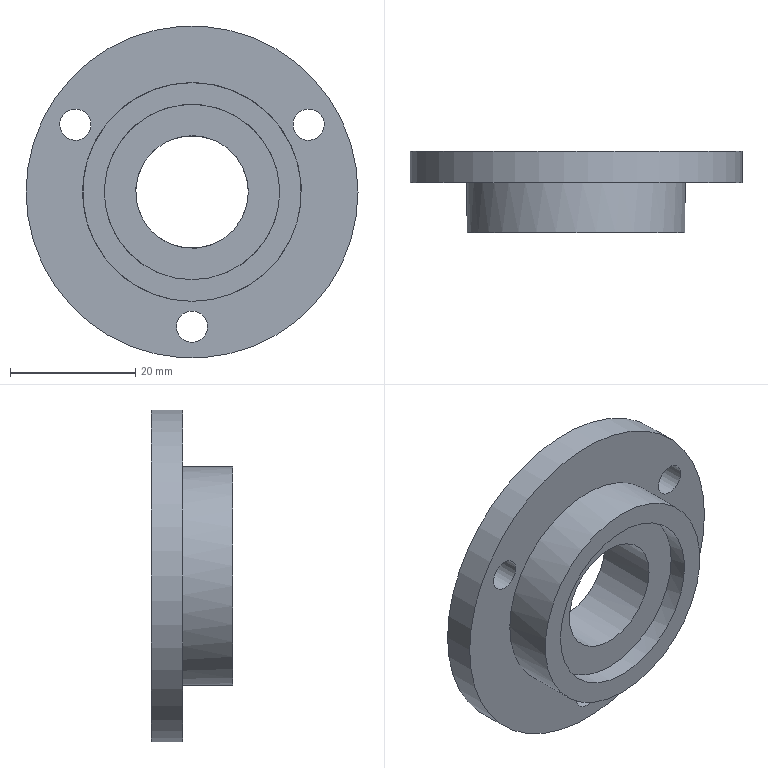Part | STEP file | YBQDJ-PD-19 | 1 solid | 11 faces | box 53 x 13 x 53 mm | volume 13997 mm3 | cylinder 7 | plane 4 | commonest cylinder face diameters 5 x3 18 x1 28 x1 34.9 x1 53 x1
STEP:
#1=CARTESIAN_POINT('',(0.,0.,0.));
#2=DIRECTION('',(0.,0.,1.));
#3=DIRECTION('',(1.,0.,0.));
#4=AXIS2_PLACEMENT_3D('',#1,#2,#3);
#5=CARTESIAN_POINT('',(-200.87,415.,131.915));
#6=VERTEX_POINT('',#5);
#7=CARTESIAN_POINT('',(-202.12,415.,129.75));
#8=DIRECTION('',(0.,1.,0.));
#9=DIRECTION('',(0.5,0.,0.866));
#10=AXIS2_PLACEMENT_3D('',#7,#8,#9);
#11=CIRCLE('',#10,2.5);
#12=CARTESIAN_POINT('',(-202.12,450.,129.75));
#13=DIRECTION('',(0.,-1.,0.));
#14=DIRECTION('',(-0.866,0.,0.5));
#15=AXIS2_PLACEMENT_3D('',#12,#13,#14);
#16=CYLINDRICAL_SURFACE('',#15,2.5);
#17=CARTESIAN_POINT('',(10.996,35.));
#18=DIRECTION('',(-1.,0.));
#19=VECTOR('',#18,1.);
#20=LINE('',#17,#19);
#21=(GEOMETRIC_REPRESENTATION_CONTEXT(2)PARAMETRIC_REPRESENTATION_CONTEXT()REPRESENTATION_CONTEXT('',''));
#22=DEFINITIONAL_REPRESENTATION('',(#20),#21);
#23=PCURVE('',#16,#22);
#24=CARTESIAN_POINT('',(-531.5,415.,22.));
#25=DIRECTION('',(0.,1.,0.));
#26=DIRECTION('',(0.,0.,-1.));
#27=AXIS2_PLACEMENT_3D('',#24,#25,#26);
#28=PLANE('',#27);
#29=CARTESIAN_POINT('',(-107.75,-329.38));
#30=DIRECTION('',(-0.866,-0.5));
#31=AXIS2_PLACEMENT_2D('',#29,#30);
#32=CIRCLE('',#31,2.5);
#33=(GEOMETRIC_REPRESENTATION_CONTEXT(2)PARAMETRIC_REPRESENTATION_CONTEXT()REPRESENTATION_CONTEXT('',''));
#34=DEFINITIONAL_REPRESENTATION('',(#32),#33);
#35=PCURVE('',#28,#34);
#36=SURFACE_CURVE('',#11,(#23,#35),.PCURVE_S1.);
#37=EDGE_CURVE('',#6,#6,#36,.T.);
#38=ORIENTED_EDGE('',*,*,#37,.T.);
#39=CARTESIAN_POINT('',(-200.87,420.,131.915));
#40=VERTEX_POINT('',#39);
#41=CARTESIAN_POINT('',(-200.87,420.,131.915));
#42=CARTESIAN_POINT('',(-200.87,415.,131.915));
#43=B_SPLINE_CURVE_WITH_KNOTS('',1,(#41,#42),.UNSPECIFIED.,.F.,.F.,(2,2),(30.,35.),.PIECEWISE_BEZIER_KNOTS.);
#44=CARTESIAN_POINT('',(4.712,0.));
#45=DIRECTION('',(0.,1.));
#46=VECTOR('',#45,1.);
#47=LINE('',#44,#46);
#48=(GEOMETRIC_REPRESENTATION_CONTEXT(2)PARAMETRIC_REPRESENTATION_CONTEXT()REPRESENTATION_CONTEXT('',''));
#49=DEFINITIONAL_REPRESENTATION('',(#47),#48);
#50=PCURVE('',#16,#49);
#51=CARTESIAN_POINT('',(10.996,0.));
#52=DIRECTION('',(0.,1.));
#53=VECTOR('',#52,1.);
#54=LINE('',#51,#53);
#55=(GEOMETRIC_REPRESENTATION_CONTEXT(2)PARAMETRIC_REPRESENTATION_CONTEXT()REPRESENTATION_CONTEXT('',''));
#56=DEFINITIONAL_REPRESENTATION('',(#54),#55);
#57=PCURVE('',#16,#56);
#58=SEAM_CURVE('',#43,(#50,#57),.PCURVE_S1.);
#59=EDGE_CURVE('',#40,#6,#58,.T.);
#60=ORIENTED_EDGE('',*,*,#59,.F.);
#61=CARTESIAN_POINT('',(-203.37,420.,127.585));
#62=VERTEX_POINT('',#61);
#63=CARTESIAN_POINT('',(-202.12,420.,129.75));
#64=DIRECTION('',(0.,1.,0.));
#65=DIRECTION('',(-0.5,0.,-0.866));
#66=AXIS2_PLACEMENT_3D('',#63,#64,#65);
#67=CIRCLE('',#66,2.5);
#68=CARTESIAN_POINT('',(7.854,30.));
#69=DIRECTION('',(-1.,0.));
#70=VECTOR('',#69,1.);
#71=LINE('',#68,#70);
#72=(GEOMETRIC_REPRESENTATION_CONTEXT(2)PARAMETRIC_REPRESENTATION_CONTEXT()REPRESENTATION_CONTEXT('',''));
#73=DEFINITIONAL_REPRESENTATION('',(#71),#72);
#74=PCURVE('',#16,#73);
#75=CARTESIAN_POINT('',(-183.5,420.,119.));
#76=DIRECTION('',(0.,-1.,0.));
#77=DIRECTION('',(-0.7071,0.,-0.7071));
#78=AXIS2_PLACEMENT_3D('',#75,#76,#77);
#79=PLANE('',#78);
#80=CARTESIAN_POINT('',(7.979,-20.12));
#81=CARTESIAN_POINT('',(9.1,-24.303));
#82=CARTESIAN_POINT('',(4.918,-23.182));
#83=CARTESIAN_POINT('',(0.735,-22.062));
#84=CARTESIAN_POINT('',(3.797,-19.));
#85=CARTESIAN_POINT('',(6.859,-15.938));
#86=CARTESIAN_POINT('',(7.979,-20.12));
#87=(BOUNDED_CURVE()B_SPLINE_CURVE(2,(#80,#81,#82,#83,#84,#85,#86),.UNSPECIFIED.,.T.,.F.)B_SPLINE_CURVE_WITH_KNOTS((1,2,2,2,2,1),(-2.094,0.,2.094,4.189,6.283,8.378),.UNSPECIFIED.)CURVE()GEOMETRIC_REPRESENTATION_ITEM()RATIONAL_B_SPLINE_CURVE((1.,0.5,1.,0.5,1.,0.5,1.))REPRESENTATION_ITEM(''));
#88=(GEOMETRIC_REPRESENTATION_CONTEXT(2)PARAMETRIC_REPRESENTATION_CONTEXT()REPRESENTATION_CONTEXT('',''));
#89=DEFINITIONAL_REPRESENTATION('',(#87),#88);
#90=PCURVE('',#79,#89);
#91=SURFACE_CURVE('',#67,(#74,#90),.PCURVE_S1.);
#92=EDGE_CURVE('',#62,#40,#91,.T.);
#93=ORIENTED_EDGE('',*,*,#92,.F.);
#94=CARTESIAN_POINT('',(-202.12,420.,129.75));
#95=DIRECTION('',(0.,1.,0.));
#96=DIRECTION('',(-0.5,0.,-0.866));
#97=AXIS2_PLACEMENT_3D('',#94,#95,#96);
#98=CIRCLE('',#97,2.5);
#99=CARTESIAN_POINT('',(14.137,30.));
#100=DIRECTION('',(-1.,0.));
#101=VECTOR('',#100,1.);
#102=LINE('',#99,#101);
#103=(GEOMETRIC_REPRESENTATION_CONTEXT(2)PARAMETRIC_REPRESENTATION_CONTEXT()REPRESENTATION_CONTEXT('',''));
#104=DEFINITIONAL_REPRESENTATION('',(#102),#103);
#105=PCURVE('',#16,#104);
#106=CARTESIAN_POINT('',(7.979,-20.12));
#107=CARTESIAN_POINT('',(9.1,-24.303));
#108=CARTESIAN_POINT('',(4.918,-23.182));
#109=CARTESIAN_POINT('',(0.735,-22.062));
#110=CARTESIAN_POINT('',(3.797,-19.));
#111=CARTESIAN_POINT('',(6.859,-15.938));
#112=CARTESIAN_POINT('',(7.979,-20.12));
#113=(BOUNDED_CURVE()B_SPLINE_CURVE(2,(#106,#107,#108,#109,#110,#111,#112),.UNSPECIFIED.,.T.,.F.)B_SPLINE_CURVE_WITH_KNOTS((1,2,2,2,2,1),(-2.094,0.,2.094,4.189,6.283,8.378),.UNSPECIFIED.)CURVE()GEOMETRIC_REPRESENTATION_ITEM()RATIONAL_B_SPLINE_CURVE((1.,0.5,1.,0.5,1.,0.5,1.))REPRESENTATION_ITEM(''));
#114=(GEOMETRIC_REPRESENTATION_CONTEXT(2)PARAMETRIC_REPRESENTATION_CONTEXT()REPRESENTATION_CONTEXT('',''));
#115=DEFINITIONAL_REPRESENTATION('',(#113),#114);
#116=PCURVE('',#79,#115);
#117=SURFACE_CURVE('',#98,(#105,#116),.PCURVE_S1.);
#118=EDGE_CURVE('',#40,#62,#117,.T.);
#119=ORIENTED_EDGE('',*,*,#118,.F.);
#120=ORIENTED_EDGE('',*,*,#59,.T.);
#121=EDGE_LOOP('',(#38,#60,#93,#119,#120));
#122=FACE_BOUND('',#121,.F.);
#123=ADVANCED_FACE('',(#122),#16,.F.);
#124=CARTESIAN_POINT('',(-163.63,415.,127.585));
#125=VERTEX_POINT('',#124);
#126=CARTESIAN_POINT('',(-164.88,415.,129.75));
#127=DIRECTION('',(0.,1.,0.));
#128=DIRECTION('',(0.5,0.,-0.866));
#129=AXIS2_PLACEMENT_3D('',#126,#127,#128);
#130=CIRCLE('',#129,2.5);
#131=CARTESIAN_POINT('',(-164.88,450.,129.75));
#132=DIRECTION('',(0.,-1.,0.));
#133=DIRECTION('',(0.866,0.,0.5));
#134=AXIS2_PLACEMENT_3D('',#131,#132,#133);
#135=CYLINDRICAL_SURFACE('',#134,2.5);
#136=CARTESIAN_POINT('',(10.996,35.));
#137=DIRECTION('',(-1.,0.));
#138=VECTOR('',#137,1.);
#139=LINE('',#136,#138);
#140=(GEOMETRIC_REPRESENTATION_CONTEXT(2)PARAMETRIC_REPRESENTATION_CONTEXT()REPRESENTATION_CONTEXT('',''));
#141=DEFINITIONAL_REPRESENTATION('',(#139),#140);
#142=PCURVE('',#135,#141);
#143=CARTESIAN_POINT('',(-107.75,-366.62));
#144=DIRECTION('',(0.866,-0.5));
#145=AXIS2_PLACEMENT_2D('',#143,#144);
#146=CIRCLE('',#145,2.5);
#147=(GEOMETRIC_REPRESENTATION_CONTEXT(2)PARAMETRIC_REPRESENTATION_CONTEXT()REPRESENTATION_CONTEXT('',''));
#148=DEFINITIONAL_REPRESENTATION('',(#146),#147);
#149=PCURVE('',#28,#148);
#150=SURFACE_CURVE('',#130,(#142,#149),.PCURVE_S1.);
#151=EDGE_CURVE('',#125,#125,#150,.T.);
#152=ORIENTED_EDGE('',*,*,#151,.T.);
#153=CARTESIAN_POINT('',(-163.63,420.,127.585));
#154=VERTEX_POINT('',#153);
#155=CARTESIAN_POINT('',(-163.63,420.,127.585));
#156=CARTESIAN_POINT('',(-163.63,415.,127.585));
#157=B_SPLINE_CURVE_WITH_KNOTS('',1,(#155,#156),.UNSPECIFIED.,.F.,.F.,(2,2),(30.,35.),.PIECEWISE_BEZIER_KNOTS.);
#158=CARTESIAN_POINT('',(4.712,0.));
#159=DIRECTION('',(0.,1.));
#160=VECTOR('',#159,1.);
#161=LINE('',#158,#160);
#162=(GEOMETRIC_REPRESENTATION_CONTEXT(2)PARAMETRIC_REPRESENTATION_CONTEXT()REPRESENTATION_CONTEXT('',''));
#163=DEFINITIONAL_REPRESENTATION('',(#161),#162);
#164=PCURVE('',#135,#163);
#165=CARTESIAN_POINT('',(10.996,0.));
#166=DIRECTION('',(0.,1.));
#167=VECTOR('',#166,1.);
#168=LINE('',#165,#167);
#169=(GEOMETRIC_REPRESENTATION_CONTEXT(2)PARAMETRIC_REPRESENTATION_CONTEXT()REPRESENTATION_CONTEXT('',''));
#170=DEFINITIONAL_REPRESENTATION('',(#168),#169);
#171=PCURVE('',#135,#170);
#172=SEAM_CURVE('',#157,(#164,#171),.PCURVE_S1.);
#173=EDGE_CURVE('',#154,#125,#172,.T.);
#174=ORIENTED_EDGE('',*,*,#173,.F.);
#175=CARTESIAN_POINT('',(-166.13,420.,131.915));
#176=VERTEX_POINT('',#175);
#177=CARTESIAN_POINT('',(-164.88,420.,129.75));
#178=DIRECTION('',(0.,1.,0.));
#179=DIRECTION('',(-0.5,0.,0.866));
#180=AXIS2_PLACEMENT_3D('',#177,#178,#179);
#181=CIRCLE('',#180,2.5);
#182=CARTESIAN_POINT('',(7.854,30.));
#183=DIRECTION('',(-1.,0.));
#184=VECTOR('',#183,1.);
#185=LINE('',#182,#184);
#186=(GEOMETRIC_REPRESENTATION_CONTEXT(2)PARAMETRIC_REPRESENTATION_CONTEXT()REPRESENTATION_CONTEXT('',''));
#187=DEFINITIONAL_REPRESENTATION('',(#185),#186);
#188=PCURVE('',#135,#187);
#189=CARTESIAN_POINT('',(-21.414,3.15));
#190=CARTESIAN_POINT('',(-25.597,4.271));
#191=CARTESIAN_POINT('',(-22.535,7.332));
#192=CARTESIAN_POINT('',(-19.473,10.394));
#193=CARTESIAN_POINT('',(-18.353,6.212));
#194=CARTESIAN_POINT('',(-17.232,2.029));
#195=CARTESIAN_POINT('',(-21.414,3.15));
#196=(BOUNDED_CURVE()B_SPLINE_CURVE(2,(#189,#190,#191,#192,#193,#194,#195),.UNSPECIFIED.,.T.,.F.)B_SPLINE_CURVE_WITH_KNOTS((1,2,2,2,2,1),(-2.094,0.,2.094,4.189,6.283,8.378),.UNSPECIFIED.)CURVE()GEOMETRIC_REPRESENTATION_ITEM()RATIONAL_B_SPLINE_CURVE((1.,0.5,1.,0.5,1.,0.5,1.))REPRESENTATION_ITEM(''));
#197=(GEOMETRIC_REPRESENTATION_CONTEXT(2)PARAMETRIC_REPRESENTATION_CONTEXT()REPRESENTATION_CONTEXT('',''));
#198=DEFINITIONAL_REPRESENTATION('',(#196),#197);
#199=PCURVE('',#79,#198);
#200=SURFACE_CURVE('',#181,(#188,#199),.PCURVE_S1.);
#201=EDGE_CURVE('',#176,#154,#200,.T.);
#202=ORIENTED_EDGE('',*,*,#201,.F.);
#203=CARTESIAN_POINT('',(-164.88,420.,129.75));
#204=DIRECTION('',(0.,1.,0.));
#205=DIRECTION('',(-0.5,0.,0.866));
#206=AXIS2_PLACEMENT_3D('',#203,#204,#205);
#207=CIRCLE('',#206,2.5);
#208=CARTESIAN_POINT('',(14.137,30.));
#209=DIRECTION('',(-1.,0.));
#210=VECTOR('',#209,1.);
#211=LINE('',#208,#210);
#212=(GEOMETRIC_REPRESENTATION_CONTEXT(2)PARAMETRIC_REPRESENTATION_CONTEXT()REPRESENTATION_CONTEXT('',''));
#213=DEFINITIONAL_REPRESENTATION('',(#211),#212);
#214=PCURVE('',#135,#213);
#215=CARTESIAN_POINT('',(-21.414,3.15));
#216=CARTESIAN_POINT('',(-25.597,4.271));
#217=CARTESIAN_POINT('',(-22.535,7.332));
#218=CARTESIAN_POINT('',(-19.473,10.394));
#219=CARTESIAN_POINT('',(-18.353,6.212));
#220=CARTESIAN_POINT('',(-17.232,2.029));
#221=CARTESIAN_POINT('',(-21.414,3.15));
#222=(BOUNDED_CURVE()B_SPLINE_CURVE(2,(#215,#216,#217,#218,#219,#220,#221),.UNSPECIFIED.,.T.,.F.)B_SPLINE_CURVE_WITH_KNOTS((1,2,2,2,2,1),(-2.094,0.,2.094,4.189,6.283,8.378),.UNSPECIFIED.)CURVE()GEOMETRIC_REPRESENTATION_ITEM()RATIONAL_B_SPLINE_CURVE((1.,0.5,1.,0.5,1.,0.5,1.))REPRESENTATION_ITEM(''));
#223=(GEOMETRIC_REPRESENTATION_CONTEXT(2)PARAMETRIC_REPRESENTATION_CONTEXT()REPRESENTATION_CONTEXT('',''));
#224=DEFINITIONAL_REPRESENTATION('',(#222),#223);
#225=PCURVE('',#79,#224);
#226=SURFACE_CURVE('',#207,(#214,#225),.PCURVE_S1.);
#227=EDGE_CURVE('',#154,#176,#226,.T.);
#228=ORIENTED_EDGE('',*,*,#227,.F.);
#229=ORIENTED_EDGE('',*,*,#173,.T.);
#230=EDGE_LOOP('',(#152,#174,#202,#228,#229));
#231=FACE_BOUND('',#230,.F.);
#232=ADVANCED_FACE('',(#231),#135,.F.);
#233=CARTESIAN_POINT('',(-210.,415.,119.));
#234=VERTEX_POINT('',#233);
#235=CARTESIAN_POINT('',(-183.5,415.,119.));
#236=DIRECTION('',(0.,1.,0.));
#237=DIRECTION('',(-1.,0.,0.));
#238=AXIS2_PLACEMENT_3D('',#235,#236,#237);
#239=CIRCLE('',#238,26.5);
#240=CARTESIAN_POINT('',(-183.5,420.,119.));
#241=DIRECTION('',(0.,-1.,0.));
#242=DIRECTION('',(-0.7071,0.,-0.7071));
#243=AXIS2_PLACEMENT_3D('',#240,#241,#242);
#244=CYLINDRICAL_SURFACE('',#243,26.5);
#245=CARTESIAN_POINT('',(11.781,5.));
#246=DIRECTION('',(-1.,0.));
#247=VECTOR('',#246,1.);
#248=LINE('',#245,#247);
#249=(GEOMETRIC_REPRESENTATION_CONTEXT(2)PARAMETRIC_REPRESENTATION_CONTEXT()REPRESENTATION_CONTEXT('',''));
#250=DEFINITIONAL_REPRESENTATION('',(#248),#249);
#251=PCURVE('',#244,#250);
#252=CARTESIAN_POINT('',(-97.,-348.));
#253=DIRECTION('',(0.,1.));
#254=AXIS2_PLACEMENT_2D('',#252,#253);
#255=CIRCLE('',#254,26.5);
#256=(GEOMETRIC_REPRESENTATION_CONTEXT(2)PARAMETRIC_REPRESENTATION_CONTEXT()REPRESENTATION_CONTEXT('',''));
#257=DEFINITIONAL_REPRESENTATION('',(#255),#256);
#258=PCURVE('',#28,#257);
#259=SURFACE_CURVE('',#239,(#251,#258),.PCURVE_S1.);
#260=EDGE_CURVE('',#234,#234,#259,.T.);
#261=ORIENTED_EDGE('',*,*,#260,.T.);
#262=CARTESIAN_POINT('',(-210.,420.,119.));
#263=VERTEX_POINT('',#262);
#264=CARTESIAN_POINT('',(-210.,420.,119.));
#265=CARTESIAN_POINT('',(-210.,415.,119.));
#266=B_SPLINE_CURVE_WITH_KNOTS('',1,(#264,#265),.UNSPECIFIED.,.F.,.F.,(2,2),(0.,5.),.PIECEWISE_BEZIER_KNOTS.);
#267=CARTESIAN_POINT('',(5.498,0.));
#268=DIRECTION('',(0.,1.));
#269=VECTOR('',#268,1.);
#270=LINE('',#267,#269);
#271=(GEOMETRIC_REPRESENTATION_CONTEXT(2)PARAMETRIC_REPRESENTATION_CONTEXT()REPRESENTATION_CONTEXT('',''));
#272=DEFINITIONAL_REPRESENTATION('',(#270),#271);
#273=PCURVE('',#244,#272);
#274=CARTESIAN_POINT('',(11.781,0.));
#275=DIRECTION('',(0.,1.));
#276=VECTOR('',#275,1.);
#277=LINE('',#274,#276);
#278=(GEOMETRIC_REPRESENTATION_CONTEXT(2)PARAMETRIC_REPRESENTATION_CONTEXT()REPRESENTATION_CONTEXT('',''));
#279=DEFINITIONAL_REPRESENTATION('',(#277),#278);
#280=PCURVE('',#244,#279);
#281=SEAM_CURVE('',#266,(#273,#280),.PCURVE_S1.);
#282=EDGE_CURVE('',#263,#234,#281,.T.);
#283=ORIENTED_EDGE('',*,*,#282,.F.);
#284=CARTESIAN_POINT('',(-157.,420.,119.));
#285=VERTEX_POINT('',#284);
#286=CARTESIAN_POINT('',(-183.5,420.,119.));
#287=DIRECTION('',(0.,1.,0.));
#288=DIRECTION('',(1.,0.,0.));
#289=AXIS2_PLACEMENT_3D('',#286,#287,#288);
#290=CIRCLE('',#289,26.5);
#291=CARTESIAN_POINT('',(8.639,0.));
#292=DIRECTION('',(-1.,0.));
#293=VECTOR('',#292,1.);
#294=LINE('',#291,#293);
#295=(GEOMETRIC_REPRESENTATION_CONTEXT(2)PARAMETRIC_REPRESENTATION_CONTEXT()REPRESENTATION_CONTEXT('',''));
#296=DEFINITIONAL_REPRESENTATION('',(#294),#295);
#297=PCURVE('',#244,#296);
#298=CARTESIAN_POINT('',(-18.738,18.738));
#299=CARTESIAN_POINT('',(13.717,51.194));
#300=CARTESIAN_POINT('',(25.597,6.859));
#301=CARTESIAN_POINT('',(37.477,-37.477));
#302=CARTESIAN_POINT('',(-6.859,-25.597));
#303=CARTESIAN_POINT('',(-51.194,-13.717));
#304=CARTESIAN_POINT('',(-18.738,18.738));
#305=(BOUNDED_CURVE()B_SPLINE_CURVE(2,(#298,#299,#300,#301,#302,#303,#304),.UNSPECIFIED.,.T.,.F.)B_SPLINE_CURVE_WITH_KNOTS((1,2,2,2,2,1),(-2.094,0.,2.094,4.189,6.283,8.378),.UNSPECIFIED.)CURVE()GEOMETRIC_REPRESENTATION_ITEM()RATIONAL_B_SPLINE_CURVE((1.,0.5,1.,0.5,1.,0.5,1.))REPRESENTATION_ITEM(''));
#306=(GEOMETRIC_REPRESENTATION_CONTEXT(2)PARAMETRIC_REPRESENTATION_CONTEXT()REPRESENTATION_CONTEXT('',''));
#307=DEFINITIONAL_REPRESENTATION('',(#305),#306);
#308=PCURVE('',#79,#307);
#309=SURFACE_CURVE('',#290,(#297,#308),.PCURVE_S1.);
#310=EDGE_CURVE('',#285,#263,#309,.T.);
#311=ORIENTED_EDGE('',*,*,#310,.F.);
#312=CARTESIAN_POINT('',(-183.5,420.,119.));
#313=DIRECTION('',(0.,1.,0.));
#314=DIRECTION('',(1.,0.,0.));
#315=AXIS2_PLACEMENT_3D('',#312,#313,#314);
#316=CIRCLE('',#315,26.5);
#317=CARTESIAN_POINT('',(14.923,0.));
#318=DIRECTION('',(-1.,0.));
#319=VECTOR('',#318,1.);
#320=LINE('',#317,#319);
#321=(GEOMETRIC_REPRESENTATION_CONTEXT(2)PARAMETRIC_REPRESENTATION_CONTEXT()REPRESENTATION_CONTEXT('',''));
#322=DEFINITIONAL_REPRESENTATION('',(#320),#321);
#323=PCURVE('',#244,#322);
#324=CARTESIAN_POINT('',(-18.738,18.738));
#325=CARTESIAN_POINT('',(13.717,51.194));
#326=CARTESIAN_POINT('',(25.597,6.859));
#327=CARTESIAN_POINT('',(37.477,-37.477));
#328=CARTESIAN_POINT('',(-6.859,-25.597));
#329=CARTESIAN_POINT('',(-51.194,-13.717));
#330=CARTESIAN_POINT('',(-18.738,18.738));
#331=(BOUNDED_CURVE()B_SPLINE_CURVE(2,(#324,#325,#326,#327,#328,#329,#330),.UNSPECIFIED.,.T.,.F.)B_SPLINE_CURVE_WITH_KNOTS((1,2,2,2,2,1),(-2.094,0.,2.094,4.189,6.283,8.378),.UNSPECIFIED.)CURVE()GEOMETRIC_REPRESENTATION_ITEM()RATIONAL_B_SPLINE_CURVE((1.,0.5,1.,0.5,1.,0.5,1.))REPRESENTATION_ITEM(''));
#332=(GEOMETRIC_REPRESENTATION_CONTEXT(2)PARAMETRIC_REPRESENTATION_CONTEXT()REPRESENTATION_CONTEXT('',''));
#333=DEFINITIONAL_REPRESENTATION('',(#331),#332);
#334=PCURVE('',#79,#333);
#335=SURFACE_CURVE('',#316,(#323,#334),.PCURVE_S1.);
#336=EDGE_CURVE('',#263,#285,#335,.T.);
#337=ORIENTED_EDGE('',*,*,#336,.F.);
#338=ORIENTED_EDGE('',*,*,#282,.T.);
#339=EDGE_LOOP('',(#261,#283,#311,#337,#338));
#340=FACE_BOUND('',#339,.T.);
#341=ADVANCED_FACE('',(#340),#244,.T.);
#342=ORIENTED_EDGE('',*,*,#92,.F.);
#343=ORIENTED_EDGE('',*,*,#118,.F.);
#344=EDGE_LOOP('',(#342,#343));
#345=FACE_BOUND('',#344,.T.);
#346=ORIENTED_EDGE('',*,*,#201,.F.);
#347=ORIENTED_EDGE('',*,*,#227,.F.);
#348=EDGE_LOOP('',(#346,#347));
#349=FACE_BOUND('',#348,.T.);
#350=CARTESIAN_POINT('',(-181.,420.,97.5));
#351=VERTEX_POINT('',#350);
#352=CARTESIAN_POINT('',(-186.,420.,97.5));
#353=VERTEX_POINT('',#352);
#354=CARTESIAN_POINT('',(-183.5,420.,97.5));
#355=DIRECTION('',(0.,1.,0.));
#356=DIRECTION('',(1.,0.,0.));
#357=AXIS2_PLACEMENT_3D('',#354,#355,#356);
#358=CIRCLE('',#357,2.5);
#359=CARTESIAN_POINT('',(13.435,16.971));
#360=CARTESIAN_POINT('',(16.497,20.032));
#361=CARTESIAN_POINT('',(17.618,15.85));
#362=CARTESIAN_POINT('',(18.738,11.667));
#363=CARTESIAN_POINT('',(14.556,12.788));
#364=CARTESIAN_POINT('',(10.373,13.909));
#365=CARTESIAN_POINT('',(13.435,16.971));
#366=(BOUNDED_CURVE()B_SPLINE_CURVE(2,(#359,#360,#361,#362,#363,#364,#365),.UNSPECIFIED.,.T.,.F.)B_SPLINE_CURVE_WITH_KNOTS((1,2,2,2,2,1),(-2.094,0.,2.094,4.189,6.283,8.378),.UNSPECIFIED.)CURVE()GEOMETRIC_REPRESENTATION_ITEM()RATIONAL_B_SPLINE_CURVE((1.,0.5,1.,0.5,1.,0.5,1.))REPRESENTATION_ITEM(''));
#367=(GEOMETRIC_REPRESENTATION_CONTEXT(2)PARAMETRIC_REPRESENTATION_CONTEXT()REPRESENTATION_CONTEXT('',''));
#368=DEFINITIONAL_REPRESENTATION('',(#366),#367);
#369=PCURVE('',#79,#368);
#370=CARTESIAN_POINT('',(-183.5,450.,97.5));
#371=DIRECTION('',(0.,-1.,0.));
#372=DIRECTION('',(0.,0.,-1.));
#373=AXIS2_PLACEMENT_3D('',#370,#371,#372);
#374=CYLINDRICAL_SURFACE('',#373,2.5);
#375=CARTESIAN_POINT('',(7.854,30.));
#376=DIRECTION('',(-1.,0.));
#377=VECTOR('',#376,1.);
#378=LINE('',#375,#377);
#379=(GEOMETRIC_REPRESENTATION_CONTEXT(2)PARAMETRIC_REPRESENTATION_CONTEXT()REPRESENTATION_CONTEXT('',''));
#380=DEFINITIONAL_REPRESENTATION('',(#378),#379);
#381=PCURVE('',#374,#380);
#382=SURFACE_CURVE('',#358,(#369,#381),.PCURVE_S1.);
#383=EDGE_CURVE('',#351,#353,#382,.T.);
#384=ORIENTED_EDGE('',*,*,#383,.F.);
#385=CARTESIAN_POINT('',(-183.5,420.,97.5));
#386=DIRECTION('',(0.,1.,0.));
#387=DIRECTION('',(1.,0.,0.));
#388=AXIS2_PLACEMENT_3D('',#385,#386,#387);
#389=CIRCLE('',#388,2.5);
#390=CARTESIAN_POINT('',(13.435,16.971));
#391=CARTESIAN_POINT('',(16.497,20.032));
#392=CARTESIAN_POINT('',(17.618,15.85));
#393=CARTESIAN_POINT('',(18.738,11.667));
#394=CARTESIAN_POINT('',(14.556,12.788));
#395=CARTESIAN_POINT('',(10.373,13.909));
#396=CARTESIAN_POINT('',(13.435,16.971));
#397=(BOUNDED_CURVE()B_SPLINE_CURVE(2,(#390,#391,#392,#393,#394,#395,#396),.UNSPECIFIED.,.T.,.F.)B_SPLINE_CURVE_WITH_KNOTS((1,2,2,2,2,1),(-2.094,0.,2.094,4.189,6.283,8.378),.UNSPECIFIED.)CURVE()GEOMETRIC_REPRESENTATION_ITEM()RATIONAL_B_SPLINE_CURVE((1.,0.5,1.,0.5,1.,0.5,1.))REPRESENTATION_ITEM(''));
#398=(GEOMETRIC_REPRESENTATION_CONTEXT(2)PARAMETRIC_REPRESENTATION_CONTEXT()REPRESENTATION_CONTEXT('',''));
#399=DEFINITIONAL_REPRESENTATION('',(#397),#398);
#400=PCURVE('',#79,#399);
#401=CARTESIAN_POINT('',(14.137,30.));
#402=DIRECTION('',(-1.,0.));
#403=VECTOR('',#402,1.);
#404=LINE('',#401,#403);
#405=(GEOMETRIC_REPRESENTATION_CONTEXT(2)PARAMETRIC_REPRESENTATION_CONTEXT()REPRESENTATION_CONTEXT('',''));
#406=DEFINITIONAL_REPRESENTATION('',(#404),#405);
#407=PCURVE('',#374,#406);
#408=SURFACE_CURVE('',#389,(#400,#407),.PCURVE_S1.);
#409=EDGE_CURVE('',#353,#351,#408,.T.);
#410=ORIENTED_EDGE('',*,*,#409,.F.);
#411=EDGE_LOOP('',(#384,#410));
#412=FACE_BOUND('',#411,.T.);
#413=ORIENTED_EDGE('',*,*,#310,.T.);
#414=ORIENTED_EDGE('',*,*,#336,.T.);
#415=EDGE_LOOP('',(#413,#414));
#416=FACE_BOUND('',#415,.T.);
#417=CARTESIAN_POINT('',(-174.5,420.,119.));
#418=VERTEX_POINT('',#417);
#419=CARTESIAN_POINT('',(-183.5,420.,119.));
#420=DIRECTION('',(0.,-1.,0.));
#421=DIRECTION('',(1.,0.,0.));
#422=AXIS2_PLACEMENT_3D('',#419,#420,#421);
#423=CIRCLE('',#422,9.);
#424=CARTESIAN_POINT('',(0.,0.));
#425=DIRECTION('',(-0.7071,0.7071));
#426=AXIS2_PLACEMENT_2D('',#424,#425);
#427=CIRCLE('',#426,9.);
#428=(GEOMETRIC_REPRESENTATION_CONTEXT(2)PARAMETRIC_REPRESENTATION_CONTEXT()REPRESENTATION_CONTEXT('',''));
#429=DEFINITIONAL_REPRESENTATION('',(#427),#428);
#430=PCURVE('',#79,#429);
#431=CARTESIAN_POINT('',(-183.5,410.,119.));
#432=DIRECTION('',(0.,1.,0.));
#433=DIRECTION('',(0.7071,0.,0.7071));
#434=AXIS2_PLACEMENT_3D('',#431,#432,#433);
#435=CYLINDRICAL_SURFACE('',#434,9.);
#436=CARTESIAN_POINT('',(7.069,10.));
#437=DIRECTION('',(-1.,0.));
#438=VECTOR('',#437,1.);
#439=LINE('',#436,#438);
#440=(GEOMETRIC_REPRESENTATION_CONTEXT(2)PARAMETRIC_REPRESENTATION_CONTEXT()REPRESENTATION_CONTEXT('',''));
#441=DEFINITIONAL_REPRESENTATION('',(#439),#440);
#442=PCURVE('',#435,#441);
#443=SURFACE_CURVE('',#423,(#430,#442),.PCURVE_S1.);
#444=EDGE_CURVE('',#418,#418,#443,.T.);
#445=ORIENTED_EDGE('',*,*,#444,.T.);
#446=EDGE_LOOP('',(#445));
#447=FACE_BOUND('',#446,.T.);
#448=ADVANCED_FACE('',(#345,#349,#412,#416,#447),#79,.F.);
#449=CARTESIAN_POINT('',(-200.95,415.,119.));
#450=VERTEX_POINT('',#449);
#451=CARTESIAN_POINT('',(-183.5,415.,101.55));
#452=VERTEX_POINT('',#451);
#453=CARTESIAN_POINT('',(-183.5,415.,119.));
#454=DIRECTION('',(0.,1.,0.));
#455=DIRECTION('',(-1.,0.,0.));
#456=AXIS2_PLACEMENT_3D('',#453,#454,#455);
#457=CIRCLE('',#456,17.45);
#458=CARTESIAN_POINT('',(-97.,-348.));
#459=DIRECTION('',(0.,1.));
#460=AXIS2_PLACEMENT_2D('',#458,#459);
#461=CIRCLE('',#460,17.45);
#462=(GEOMETRIC_REPRESENTATION_CONTEXT(2)PARAMETRIC_REPRESENTATION_CONTEXT()REPRESENTATION_CONTEXT('',''));
#463=DEFINITIONAL_REPRESENTATION('',(#461),#462);
#464=PCURVE('',#28,#463);
#465=CARTESIAN_POINT('',(-183.5,415.,119.));
#466=DIRECTION('',(0.,-1.,0.));
#467=DIRECTION('',(1.,0.,0.));
#468=AXIS2_PLACEMENT_3D('',#465,#466,#467);
#469=CYLINDRICAL_SURFACE('',#468,17.45);
#470=CARTESIAN_POINT('',(9.425,0.));
#471=DIRECTION('',(-1.,0.));
#472=VECTOR('',#471,1.);
#473=LINE('',#470,#472);
#474=(GEOMETRIC_REPRESENTATION_CONTEXT(2)PARAMETRIC_REPRESENTATION_CONTEXT()REPRESENTATION_CONTEXT('',''));
#475=DEFINITIONAL_REPRESENTATION('',(#473),#474);
#476=PCURVE('',#469,#475);
#477=SURFACE_CURVE('',#457,(#464,#476),.PCURVE_S1.);
#478=EDGE_CURVE('',#450,#452,#477,.T.);
#479=ORIENTED_EDGE('',*,*,#478,.T.);
#480=CARTESIAN_POINT('',(-183.5,415.,119.));
#481=DIRECTION('',(0.,1.,0.));
#482=DIRECTION('',(-1.,0.,0.));
#483=AXIS2_PLACEMENT_3D('',#480,#481,#482);
#484=CIRCLE('',#483,17.45);
#485=CARTESIAN_POINT('',(-97.,-348.));
#486=DIRECTION('',(0.,1.));
#487=AXIS2_PLACEMENT_2D('',#485,#486);
#488=CIRCLE('',#487,17.45);
#489=(GEOMETRIC_REPRESENTATION_CONTEXT(2)PARAMETRIC_REPRESENTATION_CONTEXT()REPRESENTATION_CONTEXT('',''));
#490=DEFINITIONAL_REPRESENTATION('',(#488),#489);
#491=PCURVE('',#28,#490);
#492=CARTESIAN_POINT('',(15.708,0.));
#493=DIRECTION('',(-1.,0.));
#494=VECTOR('',#493,1.);
#495=LINE('',#492,#494);
#496=(GEOMETRIC_REPRESENTATION_CONTEXT(2)PARAMETRIC_REPRESENTATION_CONTEXT()REPRESENTATION_CONTEXT('',''));
#497=DEFINITIONAL_REPRESENTATION('',(#495),#496);
#498=PCURVE('',#469,#497);
#499=SURFACE_CURVE('',#484,(#491,#498),.PCURVE_S1.);
#500=EDGE_CURVE('',#452,#450,#499,.T.);
#501=ORIENTED_EDGE('',*,*,#500,.T.);
#502=EDGE_LOOP('',(#479,#501));
#503=FACE_BOUND('',#502,.T.);
#504=ORIENTED_EDGE('',*,*,#37,.T.);
#505=EDGE_LOOP('',(#504));
#506=FACE_BOUND('',#505,.T.);
#507=ORIENTED_EDGE('',*,*,#151,.T.);
#508=EDGE_LOOP('',(#507));
#509=FACE_BOUND('',#508,.T.);
#510=CARTESIAN_POINT('',(-186.,415.,97.5));
#511=VERTEX_POINT('',#510);
#512=CARTESIAN_POINT('',(-183.5,415.,97.5));
#513=DIRECTION('',(0.,1.,0.));
#514=DIRECTION('',(-1.,0.,0.));
#515=AXIS2_PLACEMENT_3D('',#512,#513,#514);
#516=CIRCLE('',#515,2.5);
#517=CARTESIAN_POINT('',(-75.5,-348.));
#518=DIRECTION('',(0.,1.));
#519=AXIS2_PLACEMENT_2D('',#517,#518);
#520=CIRCLE('',#519,2.5);
#521=(GEOMETRIC_REPRESENTATION_CONTEXT(2)PARAMETRIC_REPRESENTATION_CONTEXT()REPRESENTATION_CONTEXT('',''));
#522=DEFINITIONAL_REPRESENTATION('',(#520),#521);
#523=PCURVE('',#28,#522);
#524=CARTESIAN_POINT('',(10.996,35.));
#525=DIRECTION('',(-1.,0.));
#526=VECTOR('',#525,1.);
#527=LINE('',#524,#526);
#528=(GEOMETRIC_REPRESENTATION_CONTEXT(2)PARAMETRIC_REPRESENTATION_CONTEXT()REPRESENTATION_CONTEXT('',''));
#529=DEFINITIONAL_REPRESENTATION('',(#527),#528);
#530=PCURVE('',#374,#529);
#531=SURFACE_CURVE('',#516,(#523,#530),.PCURVE_S1.);
#532=EDGE_CURVE('',#511,#511,#531,.T.);
#533=ORIENTED_EDGE('',*,*,#532,.T.);
#534=EDGE_LOOP('',(#533));
#535=FACE_BOUND('',#534,.T.);
#536=ORIENTED_EDGE('',*,*,#260,.F.);
#537=EDGE_LOOP('',(#536));
#538=FACE_BOUND('',#537,.T.);
#539=ADVANCED_FACE('',(#503,#506,#509,#535,#538),#28,.F.);
#540=CARTESIAN_POINT('',(-174.5,410.,119.));
#541=VERTEX_POINT('',#540);
#542=CARTESIAN_POINT('',(-183.5,410.,128.));
#543=VERTEX_POINT('',#542);
#544=CARTESIAN_POINT('',(-183.5,410.,119.));
#545=DIRECTION('',(0.,-1.,0.));
#546=DIRECTION('',(0.,0.,1.));
#547=AXIS2_PLACEMENT_3D('',#544,#545,#546);
#548=CIRCLE('',#547,9.);
#549=CARTESIAN_POINT('',(11.781,0.));
#550=DIRECTION('',(-1.,0.));
#551=VECTOR('',#550,1.);
#552=LINE('',#549,#551);
#553=(GEOMETRIC_REPRESENTATION_CONTEXT(2)PARAMETRIC_REPRESENTATION_CONTEXT()REPRESENTATION_CONTEXT('',''));
#554=DEFINITIONAL_REPRESENTATION('',(#552),#553);
#555=PCURVE('',#435,#554);
#556=CARTESIAN_POINT('',(-183.5,410.,119.));
#557=DIRECTION('',(0.,1.,0.));
#558=DIRECTION('',(0.,0.,1.));
#559=AXIS2_PLACEMENT_3D('',#556,#557,#558);
#560=PLANE('',#559);
#561=CARTESIAN_POINT('',(9.,0.));
#562=CARTESIAN_POINT('',(9.,-15.588));
#563=CARTESIAN_POINT('',(-4.5,-7.794));
#564=CARTESIAN_POINT('',(-18.,0.));
#565=CARTESIAN_POINT('',(-4.5,7.794));
#566=CARTESIAN_POINT('',(9.,15.588));
#567=CARTESIAN_POINT('',(9.,0.));
#568=(BOUNDED_CURVE()B_SPLINE_CURVE(2,(#561,#562,#563,#564,#565,#566,#567),.UNSPECIFIED.,.T.,.F.)B_SPLINE_CURVE_WITH_KNOTS((1,2,2,2,2,1),(-2.094,0.,2.094,4.189,6.283,8.378),.UNSPECIFIED.)CURVE()GEOMETRIC_REPRESENTATION_ITEM()RATIONAL_B_SPLINE_CURVE((1.,0.5,1.,0.5,1.,0.5,1.))REPRESENTATION_ITEM(''));
#569=(GEOMETRIC_REPRESENTATION_CONTEXT(2)PARAMETRIC_REPRESENTATION_CONTEXT()REPRESENTATION_CONTEXT('',''));
#570=DEFINITIONAL_REPRESENTATION('',(#568),#569);
#571=PCURVE('',#560,#570);
#572=SURFACE_CURVE('',#548,(#555,#571),.PCURVE_S1.);
#573=EDGE_CURVE('',#541,#543,#572,.T.);
#574=ORIENTED_EDGE('',*,*,#573,.F.);
#575=CARTESIAN_POINT('',(-174.5,410.,119.));
#576=CARTESIAN_POINT('',(-174.5,420.,119.));
#577=B_SPLINE_CURVE_WITH_KNOTS('',1,(#575,#576),.UNSPECIFIED.,.F.,.F.,(2,2),(0.,10.),.PIECEWISE_BEZIER_KNOTS.);
#578=CARTESIAN_POINT('',(7.069,0.));
#579=DIRECTION('',(0.,1.));
#580=VECTOR('',#579,1.);
#581=LINE('',#578,#580);
#582=(GEOMETRIC_REPRESENTATION_CONTEXT(2)PARAMETRIC_REPRESENTATION_CONTEXT()REPRESENTATION_CONTEXT('',''));
#583=DEFINITIONAL_REPRESENTATION('',(#581),#582);
#584=PCURVE('',#435,#583);
#585=CARTESIAN_POINT('',(0.7854,0.));
#586=DIRECTION('',(0.,1.));
#587=VECTOR('',#586,1.);
#588=LINE('',#585,#587);
#589=(GEOMETRIC_REPRESENTATION_CONTEXT(2)PARAMETRIC_REPRESENTATION_CONTEXT()REPRESENTATION_CONTEXT('',''));
#590=DEFINITIONAL_REPRESENTATION('',(#588),#589);
#591=PCURVE('',#435,#590);
#592=SEAM_CURVE('',#577,(#584,#591),.PCURVE_S1.);
#593=EDGE_CURVE('',#541,#418,#592,.T.);
#594=ORIENTED_EDGE('',*,*,#593,.T.);
#595=ORIENTED_EDGE('',*,*,#444,.T.);
#596=ORIENTED_EDGE('',*,*,#593,.F.);
#597=CARTESIAN_POINT('',(-183.5,410.,119.));
#598=DIRECTION('',(0.,-1.,0.));
#599=DIRECTION('',(0.,0.,1.));
#600=AXIS2_PLACEMENT_3D('',#597,#598,#599);
#601=CIRCLE('',#600,9.);
#602=CARTESIAN_POINT('',(5.498,0.));
#603=DIRECTION('',(-1.,0.));
#604=VECTOR('',#603,1.);
#605=LINE('',#602,#604);
#606=(GEOMETRIC_REPRESENTATION_CONTEXT(2)PARAMETRIC_REPRESENTATION_CONTEXT()REPRESENTATION_CONTEXT('',''));
#607=DEFINITIONAL_REPRESENTATION('',(#605),#606);
#608=PCURVE('',#435,#607);
#609=CARTESIAN_POINT('',(9.,0.));
#610=CARTESIAN_POINT('',(9.,-15.588));
#611=CARTESIAN_POINT('',(-4.5,-7.794));
#612=CARTESIAN_POINT('',(-18.,0.));
#613=CARTESIAN_POINT('',(-4.5,7.794));
#614=CARTESIAN_POINT('',(9.,15.588));
#615=CARTESIAN_POINT('',(9.,0.));
#616=(BOUNDED_CURVE()B_SPLINE_CURVE(2,(#609,#610,#611,#612,#613,#614,#615),.UNSPECIFIED.,.T.,.F.)B_SPLINE_CURVE_WITH_KNOTS((1,2,2,2,2,1),(-2.094,0.,2.094,4.189,6.283,8.378),.UNSPECIFIED.)CURVE()GEOMETRIC_REPRESENTATION_ITEM()RATIONAL_B_SPLINE_CURVE((1.,0.5,1.,0.5,1.,0.5,1.))REPRESENTATION_ITEM(''));
#617=(GEOMETRIC_REPRESENTATION_CONTEXT(2)PARAMETRIC_REPRESENTATION_CONTEXT()REPRESENTATION_CONTEXT('',''));
#618=DEFINITIONAL_REPRESENTATION('',(#616),#617);
#619=PCURVE('',#560,#618);
#620=SURFACE_CURVE('',#601,(#608,#619),.PCURVE_S1.);
#621=EDGE_CURVE('',#543,#541,#620,.T.);
#622=ORIENTED_EDGE('',*,*,#621,.F.);
#623=EDGE_LOOP('',(#574,#594,#595,#596,#622));
#624=FACE_BOUND('',#623,.F.);
#625=ADVANCED_FACE('',(#624),#435,.F.);
#626=ORIENTED_EDGE('',*,*,#532,.T.);
#627=CARTESIAN_POINT('',(-186.,420.,97.5));
#628=CARTESIAN_POINT('',(-186.,415.,97.5));
#629=B_SPLINE_CURVE_WITH_KNOTS('',1,(#627,#628),.UNSPECIFIED.,.F.,.F.,(2,2),(30.,35.),.PIECEWISE_BEZIER_KNOTS.);
#630=CARTESIAN_POINT('',(4.712,0.));
#631=DIRECTION('',(0.,1.));
#632=VECTOR('',#631,1.);
#633=LINE('',#630,#632);
#634=(GEOMETRIC_REPRESENTATION_CONTEXT(2)PARAMETRIC_REPRESENTATION_CONTEXT()REPRESENTATION_CONTEXT('',''));
#635=DEFINITIONAL_REPRESENTATION('',(#633),#634);
#636=PCURVE('',#374,#635);
#637=CARTESIAN_POINT('',(10.996,0.));
#638=DIRECTION('',(0.,1.));
#639=VECTOR('',#638,1.);
#640=LINE('',#637,#639);
#641=(GEOMETRIC_REPRESENTATION_CONTEXT(2)PARAMETRIC_REPRESENTATION_CONTEXT()REPRESENTATION_CONTEXT('',''));
#642=DEFINITIONAL_REPRESENTATION('',(#640),#641);
#643=PCURVE('',#374,#642);
#644=SEAM_CURVE('',#629,(#636,#643),.PCURVE_S1.);
#645=EDGE_CURVE('',#353,#511,#644,.T.);
#646=ORIENTED_EDGE('',*,*,#645,.F.);
#647=ORIENTED_EDGE('',*,*,#383,.F.);
#648=ORIENTED_EDGE('',*,*,#409,.F.);
#649=ORIENTED_EDGE('',*,*,#645,.T.);
#650=EDGE_LOOP('',(#626,#646,#647,#648,#649));
#651=FACE_BOUND('',#650,.F.);
#652=ADVANCED_FACE('',(#651),#374,.F.);
#653=CARTESIAN_POINT('',(-183.5,407.,105.));
#654=VERTEX_POINT('',#653);
#655=CARTESIAN_POINT('',(-183.5,407.,119.));
#656=DIRECTION('',(0.,1.,0.));
#657=DIRECTION('',(0.,0.,-1.));
#658=AXIS2_PLACEMENT_3D('',#655,#656,#657);
#659=CIRCLE('',#658,14.);
#660=CARTESIAN_POINT('',(-183.5,407.,119.));
#661=DIRECTION('',(0.,-1.,0.));
#662=DIRECTION('',(0.,0.,-1.));
#663=AXIS2_PLACEMENT_3D('',#660,#661,#662);
#664=PLANE('',#663);
#665=CARTESIAN_POINT('',(14.,0.));
#666=CARTESIAN_POINT('',(14.,-24.249));
#667=CARTESIAN_POINT('',(-7.,-12.124));
#668=CARTESIAN_POINT('',(-28.,0.));
#669=CARTESIAN_POINT('',(-7.,12.124));
#670=CARTESIAN_POINT('',(14.,24.249));
#671=CARTESIAN_POINT('',(14.,0.));
#672=(BOUNDED_CURVE()B_SPLINE_CURVE(2,(#665,#666,#667,#668,#669,#670,#671),.UNSPECIFIED.,.T.,.F.)B_SPLINE_CURVE_WITH_KNOTS((1,2,2,2,2,1),(-2.094,0.,2.094,4.189,6.283,8.378),.UNSPECIFIED.)CURVE()GEOMETRIC_REPRESENTATION_ITEM()RATIONAL_B_SPLINE_CURVE((1.,0.5,1.,0.5,1.,0.5,1.))REPRESENTATION_ITEM(''));
#673=(GEOMETRIC_REPRESENTATION_CONTEXT(2)PARAMETRIC_REPRESENTATION_CONTEXT()REPRESENTATION_CONTEXT('',''));
#674=DEFINITIONAL_REPRESENTATION('',(#672),#673);
#675=PCURVE('',#664,#674);
#676=CARTESIAN_POINT('',(-183.5,411.,119.));
#677=DIRECTION('',(0.,-1.,0.));
#678=DIRECTION('',(0.,0.,-1.));
#679=AXIS2_PLACEMENT_3D('',#676,#677,#678);
#680=CYLINDRICAL_SURFACE('',#679,14.);
#681=CARTESIAN_POINT('',(6.283,4.));
#682=DIRECTION('',(-1.,0.));
#683=VECTOR('',#682,1.);
#684=LINE('',#681,#683);
#685=(GEOMETRIC_REPRESENTATION_CONTEXT(2)PARAMETRIC_REPRESENTATION_CONTEXT()REPRESENTATION_CONTEXT('',''));
#686=DEFINITIONAL_REPRESENTATION('',(#684),#685);
#687=PCURVE('',#680,#686);
#688=SURFACE_CURVE('',#659,(#675,#687),.PCURVE_S1.);
#689=EDGE_CURVE('',#654,#654,#688,.T.);
#690=ORIENTED_EDGE('',*,*,#689,.T.);
#691=EDGE_LOOP('',(#690));
#692=FACE_BOUND('',#691,.T.);
#693=CARTESIAN_POINT('',(-183.5,407.,101.55));
#694=VERTEX_POINT('',#693);
#695=CARTESIAN_POINT('',(-183.5,407.,119.));
#696=DIRECTION('',(0.,1.,0.));
#697=DIRECTION('',(0.,0.,-1.));
#698=AXIS2_PLACEMENT_3D('',#695,#696,#697);
#699=CIRCLE('',#698,17.45);
#700=CARTESIAN_POINT('',(17.45,0.));
#701=CARTESIAN_POINT('',(17.45,-30.224));
#702=CARTESIAN_POINT('',(-8.725,-15.112));
#703=CARTESIAN_POINT('',(-34.9,0.));
#704=CARTESIAN_POINT('',(-8.725,15.112));
#705=CARTESIAN_POINT('',(17.45,30.224));
#706=CARTESIAN_POINT('',(17.45,0.));
#707=(BOUNDED_CURVE()B_SPLINE_CURVE(2,(#700,#701,#702,#703,#704,#705,#706),.UNSPECIFIED.,.T.,.F.)B_SPLINE_CURVE_WITH_KNOTS((1,2,2,2,2,1),(-2.094,0.,2.094,4.189,6.283,8.378),.UNSPECIFIED.)CURVE()GEOMETRIC_REPRESENTATION_ITEM()RATIONAL_B_SPLINE_CURVE((1.,0.5,1.,0.5,1.,0.5,1.))REPRESENTATION_ITEM(''));
#708=(GEOMETRIC_REPRESENTATION_CONTEXT(2)PARAMETRIC_REPRESENTATION_CONTEXT()REPRESENTATION_CONTEXT('',''));
#709=DEFINITIONAL_REPRESENTATION('',(#707),#708);
#710=PCURVE('',#664,#709);
#711=CARTESIAN_POINT('',(10.996,8.));
#712=DIRECTION('',(-1.,0.));
#713=VECTOR('',#712,1.);
#714=LINE('',#711,#713);
#715=(GEOMETRIC_REPRESENTATION_CONTEXT(2)PARAMETRIC_REPRESENTATION_CONTEXT()REPRESENTATION_CONTEXT('',''));
#716=DEFINITIONAL_REPRESENTATION('',(#714),#715);
#717=PCURVE('',#469,#716);
#718=SURFACE_CURVE('',#699,(#710,#717),.PCURVE_S1.);
#719=EDGE_CURVE('',#694,#694,#718,.T.);
#720=ORIENTED_EDGE('',*,*,#719,.F.);
#721=EDGE_LOOP('',(#720));
#722=FACE_BOUND('',#721,.T.);
#723=ADVANCED_FACE('',(#692,#722),#664,.T.);
#724=ORIENTED_EDGE('',*,*,#500,.F.);
#725=CARTESIAN_POINT('',(-183.5,415.,101.55));
#726=CARTESIAN_POINT('',(-183.5,407.,101.55));
#727=B_SPLINE_CURVE_WITH_KNOTS('',1,(#725,#726),.UNSPECIFIED.,.F.,.F.,(2,2),(0.,8.),.PIECEWISE_BEZIER_KNOTS.);
#728=CARTESIAN_POINT('',(10.996,0.));
#729=DIRECTION('',(0.,1.));
#730=VECTOR('',#729,1.);
#731=LINE('',#728,#730);
#732=(GEOMETRIC_REPRESENTATION_CONTEXT(2)PARAMETRIC_REPRESENTATION_CONTEXT()REPRESENTATION_CONTEXT('',''));
#733=DEFINITIONAL_REPRESENTATION('',(#731),#732);
#734=PCURVE('',#469,#733);
#735=CARTESIAN_POINT('',(4.712,0.));
#736=DIRECTION('',(0.,1.));
#737=VECTOR('',#736,1.);
#738=LINE('',#735,#737);
#739=(GEOMETRIC_REPRESENTATION_CONTEXT(2)PARAMETRIC_REPRESENTATION_CONTEXT()REPRESENTATION_CONTEXT('',''));
#740=DEFINITIONAL_REPRESENTATION('',(#738),#739);
#741=PCURVE('',#469,#740);
#742=SEAM_CURVE('',#727,(#734,#741),.PCURVE_S1.);
#743=EDGE_CURVE('',#452,#694,#742,.T.);
#744=ORIENTED_EDGE('',*,*,#743,.T.);
#745=ORIENTED_EDGE('',*,*,#719,.T.);
#746=ORIENTED_EDGE('',*,*,#743,.F.);
#747=ORIENTED_EDGE('',*,*,#478,.F.);
#748=EDGE_LOOP('',(#724,#744,#745,#746,#747));
#749=FACE_BOUND('',#748,.T.);
#750=ADVANCED_FACE('',(#749),#469,.T.);
#751=CARTESIAN_POINT('',(-183.5,410.,133.));
#752=VERTEX_POINT('',#751);
#753=CARTESIAN_POINT('',(-183.5,410.,105.));
#754=VERTEX_POINT('',#753);
#755=CARTESIAN_POINT('',(-183.5,410.,119.));
#756=DIRECTION('',(0.,-1.,0.));
#757=DIRECTION('',(0.,0.,1.));
#758=AXIS2_PLACEMENT_3D('',#755,#756,#757);
#759=CIRCLE('',#758,14.);
#760=CARTESIAN_POINT('',(14.,0.));
#761=CARTESIAN_POINT('',(14.,-24.249));
#762=CARTESIAN_POINT('',(-7.,-12.124));
#763=CARTESIAN_POINT('',(-28.,0.));
#764=CARTESIAN_POINT('',(-7.,12.124));
#765=CARTESIAN_POINT('',(14.,24.249));
#766=CARTESIAN_POINT('',(14.,0.));
#767=(BOUNDED_CURVE()B_SPLINE_CURVE(2,(#760,#761,#762,#763,#764,#765,#766),.UNSPECIFIED.,.T.,.F.)B_SPLINE_CURVE_WITH_KNOTS((1,2,2,2,2,1),(-2.094,0.,2.094,4.189,6.283,8.378),.UNSPECIFIED.)CURVE()GEOMETRIC_REPRESENTATION_ITEM()RATIONAL_B_SPLINE_CURVE((1.,0.5,1.,0.5,1.,0.5,1.))REPRESENTATION_ITEM(''));
#768=(GEOMETRIC_REPRESENTATION_CONTEXT(2)PARAMETRIC_REPRESENTATION_CONTEXT()REPRESENTATION_CONTEXT('',''));
#769=DEFINITIONAL_REPRESENTATION('',(#767),#768);
#770=PCURVE('',#560,#769);
#771=CARTESIAN_POINT('',(3.142,1.));
#772=DIRECTION('',(1.,0.));
#773=VECTOR('',#772,1.);
#774=LINE('',#771,#773);
#775=(GEOMETRIC_REPRESENTATION_CONTEXT(2)PARAMETRIC_REPRESENTATION_CONTEXT()REPRESENTATION_CONTEXT('',''));
#776=DEFINITIONAL_REPRESENTATION('',(#774),#775);
#777=PCURVE('',#680,#776);
#778=SURFACE_CURVE('',#759,(#770,#777),.PCURVE_S1.);
#779=EDGE_CURVE('',#752,#754,#778,.T.);
#780=ORIENTED_EDGE('',*,*,#779,.T.);
#781=CARTESIAN_POINT('',(-183.5,410.,119.));
#782=DIRECTION('',(0.,-1.,0.));
#783=DIRECTION('',(0.,0.,1.));
#784=AXIS2_PLACEMENT_3D('',#781,#782,#783);
#785=CIRCLE('',#784,14.);
#786=CARTESIAN_POINT('',(14.,0.));
#787=CARTESIAN_POINT('',(14.,-24.249));
#788=CARTESIAN_POINT('',(-7.,-12.124));
#789=CARTESIAN_POINT('',(-28.,0.));
#790=CARTESIAN_POINT('',(-7.,12.124));
#791=CARTESIAN_POINT('',(14.,24.249));
#792=CARTESIAN_POINT('',(14.,0.));
#793=(BOUNDED_CURVE()B_SPLINE_CURVE(2,(#786,#787,#788,#789,#790,#791,#792),.UNSPECIFIED.,.T.,.F.)B_SPLINE_CURVE_WITH_KNOTS((1,2,2,2,2,1),(-2.094,0.,2.094,4.189,6.283,8.378),.UNSPECIFIED.)CURVE()GEOMETRIC_REPRESENTATION_ITEM()RATIONAL_B_SPLINE_CURVE((1.,0.5,1.,0.5,1.,0.5,1.))REPRESENTATION_ITEM(''));
#794=(GEOMETRIC_REPRESENTATION_CONTEXT(2)PARAMETRIC_REPRESENTATION_CONTEXT()REPRESENTATION_CONTEXT('',''));
#795=DEFINITIONAL_REPRESENTATION('',(#793),#794);
#796=PCURVE('',#560,#795);
#797=CARTESIAN_POINT('',(-3.142,1.));
#798=DIRECTION('',(1.,0.));
#799=VECTOR('',#798,1.);
#800=LINE('',#797,#799);
#801=(GEOMETRIC_REPRESENTATION_CONTEXT(2)PARAMETRIC_REPRESENTATION_CONTEXT()REPRESENTATION_CONTEXT('',''));
#802=DEFINITIONAL_REPRESENTATION('',(#800),#801);
#803=PCURVE('',#680,#802);
#804=SURFACE_CURVE('',#785,(#796,#803),.PCURVE_S1.);
#805=EDGE_CURVE('',#754,#752,#804,.T.);
#806=ORIENTED_EDGE('',*,*,#805,.T.);
#807=EDGE_LOOP('',(#780,#806));
#808=FACE_BOUND('',#807,.T.);
#809=ORIENTED_EDGE('',*,*,#621,.F.);
#810=ORIENTED_EDGE('',*,*,#573,.F.);
#811=EDGE_LOOP('',(#809,#810));
#812=FACE_BOUND('',#811,.T.);
#813=ADVANCED_FACE('',(#808,#812),#560,.F.);
#814=ORIENTED_EDGE('',*,*,#779,.T.);
#815=CARTESIAN_POINT('',(-183.5,410.,105.));
#816=CARTESIAN_POINT('',(-183.5,407.,105.));
#817=B_SPLINE_CURVE_WITH_KNOTS('',1,(#815,#816),.UNSPECIFIED.,.F.,.F.,(2,2),(1.,4.),.PIECEWISE_BEZIER_KNOTS.);
#818=CARTESIAN_POINT('',(6.283,0.));
#819=DIRECTION('',(0.,1.));
#820=VECTOR('',#819,1.);
#821=LINE('',#818,#820);
#822=(GEOMETRIC_REPRESENTATION_CONTEXT(2)PARAMETRIC_REPRESENTATION_CONTEXT()REPRESENTATION_CONTEXT('',''));
#823=DEFINITIONAL_REPRESENTATION('',(#821),#822);
#824=PCURVE('',#680,#823);
#825=CARTESIAN_POINT('',(0.,0.));
#826=DIRECTION('',(0.,1.));
#827=VECTOR('',#826,1.);
#828=LINE('',#825,#827);
#829=(GEOMETRIC_REPRESENTATION_CONTEXT(2)PARAMETRIC_REPRESENTATION_CONTEXT()REPRESENTATION_CONTEXT('',''));
#830=DEFINITIONAL_REPRESENTATION('',(#828),#829);
#831=PCURVE('',#680,#830);
#832=SEAM_CURVE('',#817,(#824,#831),.PCURVE_S1.);
#833=EDGE_CURVE('',#754,#654,#832,.T.);
#834=ORIENTED_EDGE('',*,*,#833,.T.);
#835=ORIENTED_EDGE('',*,*,#689,.T.);
#836=ORIENTED_EDGE('',*,*,#833,.F.);
#837=ORIENTED_EDGE('',*,*,#805,.T.);
#838=EDGE_LOOP('',(#814,#834,#835,#836,#837));
#839=FACE_BOUND('',#838,.F.);
#840=ADVANCED_FACE('',(#839),#680,.F.);
#841=CLOSED_SHELL('',(#123,#232,#341,#448,#539,#625,#652,#723,#750,#813,#840));
#842=MANIFOLD_SOLID_BREP('',#841);
#843=(LENGTH_UNIT()NAMED_UNIT(*)SI_UNIT(.MILLI.,.METRE.));
#844=UNCERTAINTY_MEASURE_WITH_UNIT(LENGTH_MEASURE(0.000005),#843,'','');
#845=(NAMED_UNIT(*)PLANE_ANGLE_UNIT()SI_UNIT($,.RADIAN.));
#846=(NAMED_UNIT(*)SI_UNIT($,.STERADIAN.)SOLID_ANGLE_UNIT());
#847=(GEOMETRIC_REPRESENTATION_CONTEXT(3)GLOBAL_UNCERTAINTY_ASSIGNED_CONTEXT((#844))GLOBAL_UNIT_ASSIGNED_CONTEXT((#843,#845,#846))REPRESENTATION_CONTEXT('',''));
#848=ADVANCED_BREP_SHAPE_REPRESENTATION('',(#4,#842),#847);